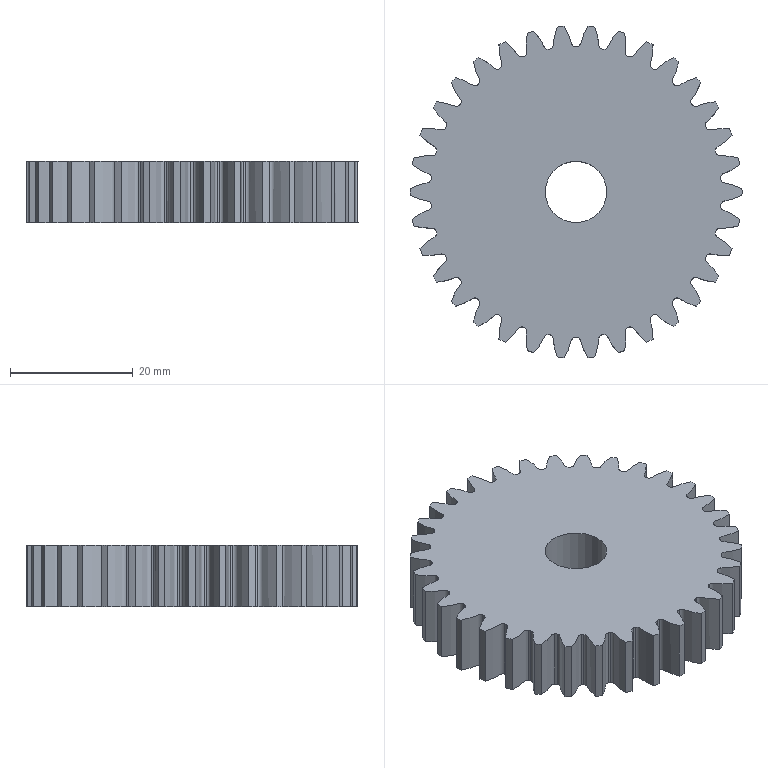Part | STEP file | Cylindrical gear 34_1.5 | 1 solid | 139 faces | box 54 x 53.862 x 10 mm | volume 19460 mm3 | cylinder 69 | spline 68 | plane 2 | commonest cylinder face diameters 47.25 x34 54 x34 10 x1